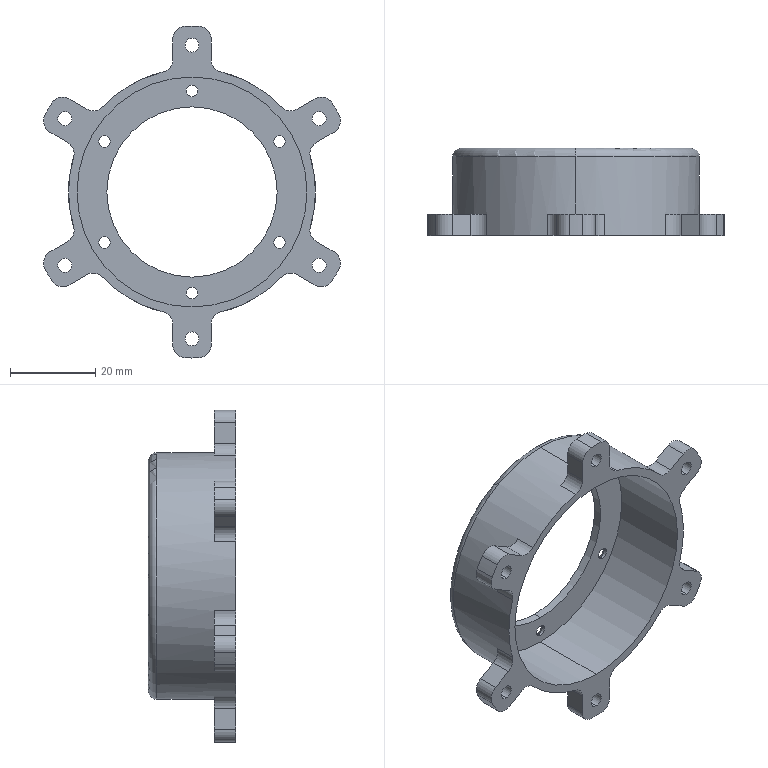Part | SolidWorks | features Fillet 2, HoleWzd 2, ICE 2, Extrusion 1 | 1 solid | 100 faces | box 69.8 x 20.5 x 78 mm | volume 11428 mm3 | cylinder 65 | plane 21 | cone 12 | torus 2 | commonest cylinder face diameters 6 x28 2.7 x12 3.3 x12 78 x7 40 x2 54 x2